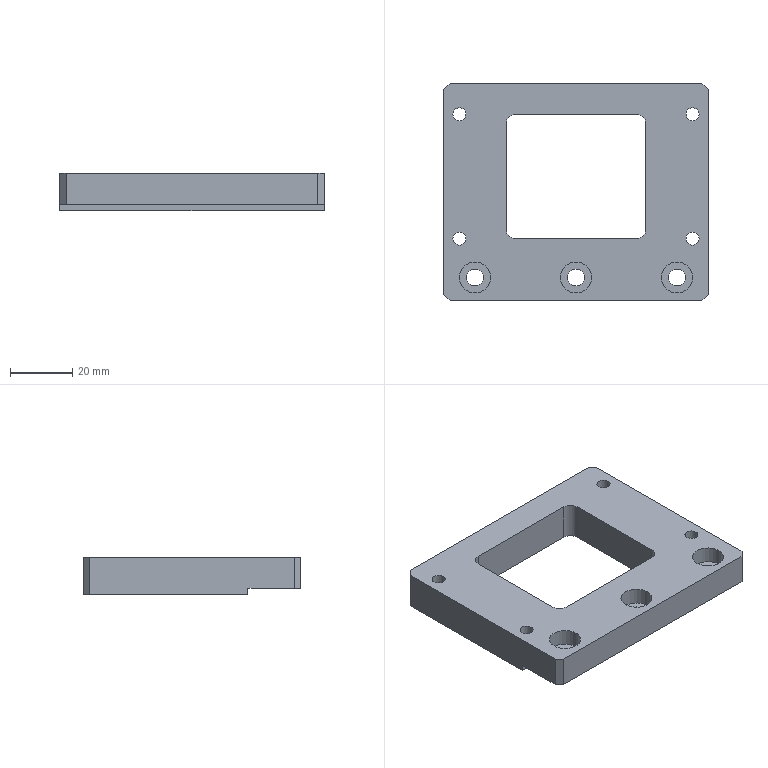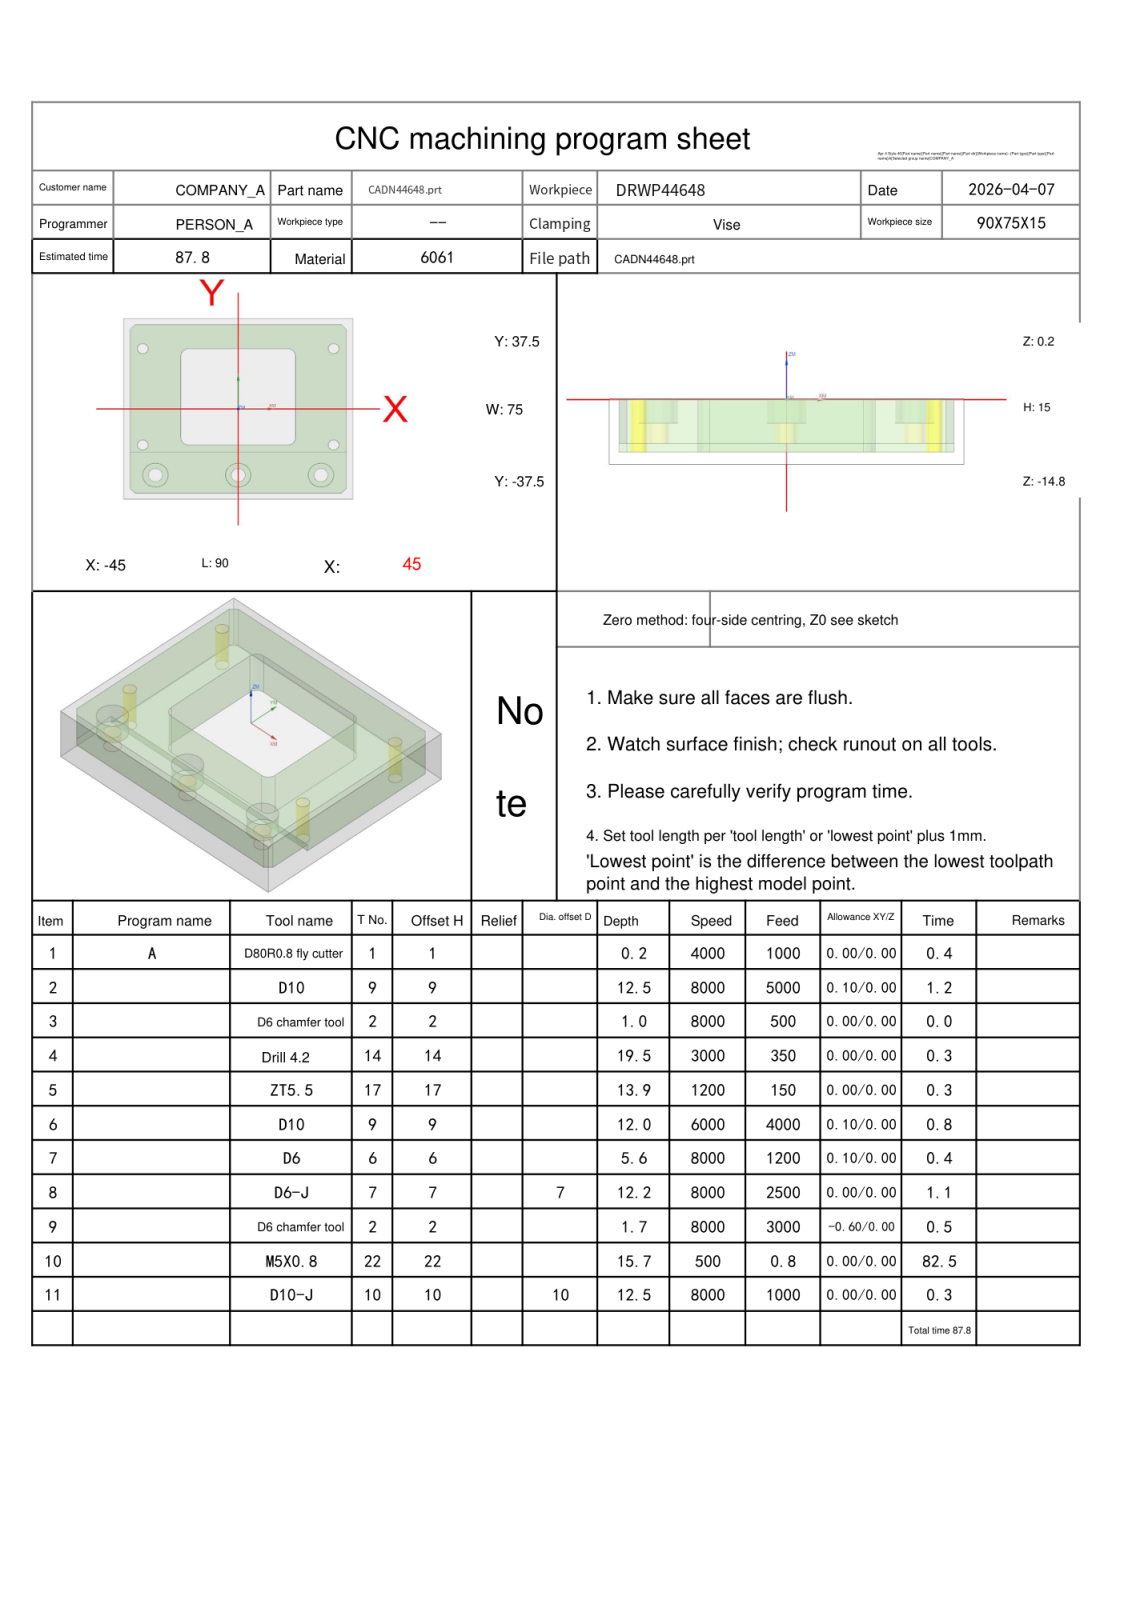NC program | NX | posted by the shop | part box 85 x 70 x 12 mm
Lines 5512 to 5800 of 5800:
N9 T02 M06
(D6 chamfer tool  D=6. R=0. H=02 ce=0.00 di=0.00)
G00 G90 G54 X.25 Y-37.128 M03 S8000
G43 H02 Z20.
M08
Z2.099
G01 Z-1.5 F3000.
G03 X.33 Y-36.828 I-.52 J.3
X.03 Y-36.308 I-.6 J0.0
G01 X0.0 Y-36.3
X-40.5
X-40.754 Y-36.275
X-40.997 Y-36.201
X-41.222 Y-36.081
X-41.419 Y-35.919
X-43.419 Y-33.919
X-43.581 Y-33.722
X-43.701 Y-33.497
X-43.775 Y-33.254
X-43.8 Y-33.
Y33.
X-43.775 Y33.254
X-43.701 Y33.497
X-43.581 Y33.722
X-43.419 Y33.919
X-41.419 Y35.919
X-41.222 Y36.081
X-40.997 Y36.201
X-40.754 Y36.275
X-40.5 Y36.3
X40.5
X40.754 Y36.275
X40.997 Y36.201
X41.222 Y36.081
X41.419 Y35.919
X43.419 Y33.919
X43.581 Y33.722
X43.701 Y33.497
X43.775 Y33.254
X43.8 Y33.
Y-33.
X43.775 Y-33.254
X43.701 Y-33.497
X43.581 Y-33.722
X43.419 Y-33.919
X41.419 Y-35.919
X41.222 Y-36.081
X40.997 Y-36.201
X40.754 Y-36.275
X40.5 Y-36.3
X0.0
X-.03 Y-36.308
G03 X-.33 Y-36.828 I.3 J-.52
X-.25 Y-37.128 I.6 J0.0
G01 Z2.099
G00 Z20.
Y-12.872
Z2.099
G01 Z-1.5
G03 X-.33 Y-13.172 I.52 J-.3
X-.03 Y-13.692 I.6 J0.0
G01 X0.0 Y-13.7
X19.5
G03 X21.2 Y-12. I0.0 J1.7
G01 Y22.
G03 X19.5 Y23.7 I-1.7 J0.0
G01 X-19.5
G03 X-21.2 Y22. I0.0 J-1.7
G01 Y-12.
G03 X-19.5 Y-13.7 I1.7 J0.0
G01 X0.0
X.03 Y-13.692
G03 X.33 Y-13.172 I-.3 J.52
X.25 Y-12.872 I-.6 J0.0
G01 Z2.099
G00 Z20.
G00 G90 X37.407 Y25.694 M03 S8000
Z20.
Z-.5
G01 Z-1. F500.
X37.3 Y26.5
G03 X35.8 Y25. I0.0 J-1.5
X37.5 Y23.3 I1.7 J0.0
X39.2 Y25. I0.0 J1.7
X37.5 Y26.7 I-1.7 J0.0
X35.8 Y25. I0.0 J-1.7
X37.3 Y23.5 I1.5 J0.0
G01 X37.407 Y24.306
Z-.5
G00 Z20.
Y-14.306
Z-.5
G01 Z-1.
X37.3 Y-13.5
G03 X35.8 Y-15. I0.0 J-1.5
X37.5 Y-16.7 I1.7 J0.0
X39.2 Y-15. I0.0 J1.7
X37.5 Y-13.3 I-1.7 J0.0
X35.8 Y-15. I0.0 J-1.7
X37.3 Y-16.5 I1.5 J0.0
G01 X37.407 Y-15.694
Z-.5
G00 Z20.
X-37.593 Y-14.306
Z-.5
G01 Z-1.
X-37.7 Y-13.5
G03 X-39.2 Y-15. I0.0 J-1.5
X-37.5 Y-16.7 I1.7 J0.0
X-35.8 Y-15. I0.0 J1.7
X-37.5 Y-13.3 I-1.7 J0.0
X-39.2 Y-15. I0.0 J-1.7
X-37.7 Y-16.5 I1.5 J0.0
G01 X-37.593 Y-15.694
Z-.5
G00 Z20.
Y25.694
Z-.5
G01 Z-1.
X-37.7 Y26.5
G03 X-39.2 Y25. I0.0 J-1.5
X-37.5 Y23.3 I1.7 J0.0
X-35.8 Y25. I0.0 J1.7
X-37.5 Y26.7 I-1.7 J0.0
X-39.2 Y25. I0.0 J-1.7
X-37.7 Y23.5 I1.5 J0.0
G01 X-37.593 Y24.306
Z-.5
G00 Z20.
G00 G90 X29.846 Y-30.886 M03 S8000
Z20.
Z2.5
G01 X29.855 Y-30.894 Z2.495 F800.
X30.211 Y-31.144 Z2.337
X30.489 Y-31.304 Z2.22
X30.883 Y-31.488 Z2.062
X31.293 Y-31.63 Z1.904
X31.716 Y-31.731 Z1.746
X32.146 Y-31.788 Z1.588
X32.58 Y-31.802 Z1.43
X33.014 Y-31.772 Z1.272
X33.442 Y-31.699 Z1.114
X33.86 Y-31.582 Z.956
X34.265 Y-31.424 Z.797
X34.652 Y-31.227 Z.639
X35.016 Y-30.991 Z.481
X35.355 Y-30.719 Z.323
X35.665 Y-30.415 Z.165
X35.943 Y-30.081 Z.007
X36.186 Y-29.721 Z-.151
X36.391 Y-29.338 Z-.309
X36.556 Y-28.936 Z-.467
X36.68 Y-28.52 Z-.625
X36.762 Y-28.093 Z-.783
X36.8 Y-27.661 Z-.942
Y-27.5 Z-1.
G03 X32.5 Y-23.2 I-4.3 J0.0
X28.2 Y-27.5 I0.0 J-4.3
X32.5 Y-31.8 I4.3 J0.0
X36.8 Y-27.5 I0.0 J4.3
X36.771 Y-27.001 I-4.3 J0.0
G01 Z1.5
G00 Z20.
X-2.654 Y-30.886
Z2.5
G01 X-2.645 Y-30.894 Z2.495
X-2.289 Y-31.144 Z2.337
X-2.011 Y-31.304 Z2.22
X-1.617 Y-31.488 Z2.062
X-1.207 Y-31.63 Z1.904
X-.784 Y-31.731 Z1.746
X-.354 Y-31.788 Z1.588
X.08 Y-31.802 Z1.43
X.514 Y-31.772 Z1.272
X.942 Y-31.699 Z1.114
X1.36 Y-31.582 Z.956
X1.765 Y-31.424 Z.797
X2.152 Y-31.227 Z.639
X2.516 Y-30.991 Z.481
X2.855 Y-30.719 Z.323
X3.165 Y-30.415 Z.165
X3.443 Y-30.081 Z.007
X3.686 Y-29.721 Z-.151
X3.891 Y-29.338 Z-.309
X4.056 Y-28.936 Z-.467
X4.18 Y-28.52 Z-.625
X4.262 Y-28.093 Z-.783
X4.3 Y-27.661 Z-.942
Y-27.5 Z-1.
G03 X0.0 Y-23.2 I-4.3 J0.0
X-4.3 Y-27.5 I0.0 J-4.3
X0.0 Y-31.8 I4.3 J0.0
X4.3 Y-27.5 I0.0 J4.3
X4.271 Y-27.001 I-4.3 J0.0
G01 Z1.5
G00 Z20.
X-35.154 Y-30.886
Z2.5
G01 X-35.145 Y-30.894 Z2.495
X-34.789 Y-31.144 Z2.337
X-34.511 Y-31.304 Z2.22
X-34.117 Y-31.488 Z2.062
X-33.707 Y-31.63 Z1.904
X-33.284 Y-31.731 Z1.746
X-32.854 Y-31.788 Z1.588
X-32.42 Y-31.802 Z1.43
X-31.986 Y-31.772 Z1.272
X-31.558 Y-31.699 Z1.114
X-31.14 Y-31.582 Z.956
X-30.735 Y-31.424 Z.797
X-30.349 Y-31.227 Z.639
X-29.984 Y-30.991 Z.481
X-29.645 Y-30.719 Z.323
X-29.335 Y-30.415 Z.165
X-29.057 Y-30.081 Z.007
X-28.814 Y-29.721 Z-.151
X-28.609 Y-29.338 Z-.309
X-28.444 Y-28.936 Z-.467
X-28.32 Y-28.52 Z-.625
X-28.238 Y-28.093 Z-.783
X-28.2 Y-27.661 Z-.942
Y-27.5 Z-1.
G03 X-32.5 Y-23.2 I-4.3 J0.0
X-36.8 Y-27.5 I0.0 J-4.3
X-32.5 Y-31.8 I4.3 J0.0
X-28.2 Y-27.5 I0.0 J4.3
X-28.229 Y-27.001 I-4.3 J0.0
G01 Z1.5
G00 Z20.
G91 G28 Z0.0
M05
M09
G91 G28 Z0.0
M01
N10 T22 M06
(M5X0.8 D=4.2 DR_a=180 H=22)
G00 G90 G54 X37.5 Y25. M03 S500
G43 H22 Z20.
M08
G95
G98 G84 X37.5 Y25. Z-15.5 R1. F.8 Q3.
Y-15.
X-37.5
Y25.
G80
G94
G00 Z20.
G91 G28 Z0.0
M05
M09
G91 G28 Z0.0
M01
N11 T10 M06
(D10-J  D=10. R=0. H=10 ce=0.00 di=0.00)
G00 G90 G54 X41.513 Y-41.116 M03 S8000
G43 H10 Z20.
M08
Z-11.8
G01 Z-12.3 F1000.
G41 D10
X41.497 Y-40.917
G03 X40.5 Y-40. I-.997 J-.083
G01 X-40.5
G02 X-44.036 Y-38.536 I0.0 J5.
G01 X-46.036 Y-36.536
G02 X-47.5 Y-33. I3.536 J3.536
G01 Y33.
G02 X-46.036 Y36.536 I5. J0.0
G01 X-44.036 Y38.536
G02 X-40.5 Y40. I3.536 J-3.536
G01 X40.5
G02 X44.036 Y38.536 I0.0 J-5.
G01 X46.036 Y36.536
G02 X47.5 Y33. I-3.536 J-3.536
G01 Y-33.
G02 X46.036 Y-36.536 I-5. J0.0
G01 X44.036 Y-38.536
G02 X40.5 Y-40. I-3.536 J3.536
G01 X40.
G03 X39. Y-41. I0.0 J-1.
G01 G40 Y-41.2
Z-11.8
G00 Z20.
M05
M09
G91 G28 Z0.0
G91 G28 Y0.0
M30
%